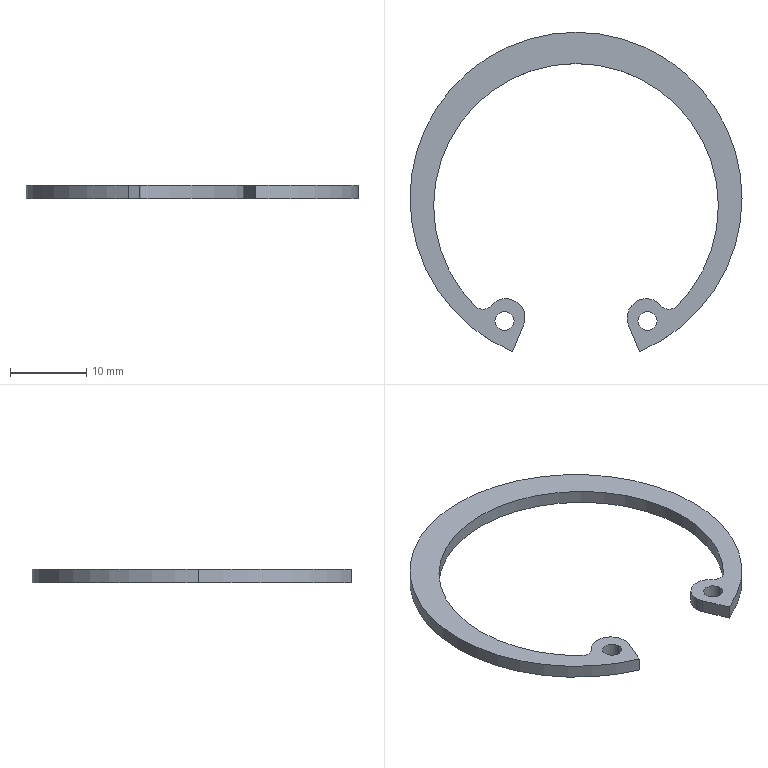Part | SolidWorks | features Extrusion 1 | 1 solid | 19 faces | box 43.5 x 41.844 x 1.75 mm | volume 670.953 mm3 | cylinder 15 | plane 4 | commonest cylinder face diameters 2.5 x4 5 x3 37.3 x3 43.5 x3 3 x2
STEP:
#1=CARTESIAN_POINT('',(8.113,-16.072,1.75));
#2=VERTEX_POINT('',#1);
#3=CARTESIAN_POINT('',(10.613,-16.072,1.75));
#4=VERTEX_POINT('',#3);
#5=CARTESIAN_POINT('',(9.363,-16.072,1.75));
#6=DIRECTION('',(0.,0.,1.));
#7=DIRECTION('',(-1.,0.,0.));
#8=AXIS2_PLACEMENT_3D('',#5,#6,#7);
#9=CIRCLE('',#8,1.25);
#10=EDGE_CURVE('',#2,#4,#9,.T.);
#11=ORIENTED_EDGE('',*,*,#10,.T.);
#12=CARTESIAN_POINT('',(10.613,-16.072,0.));
#13=VERTEX_POINT('',#12);
#14=CARTESIAN_POINT('',(10.613,-16.072,1.75));
#15=DIRECTION('',(0.,0.,-1.));
#16=VECTOR('',#15,1000.);
#17=LINE('',#14,#16);
#18=EDGE_CURVE('',#4,#13,#17,.T.);
#19=ORIENTED_EDGE('',*,*,#18,.T.);
#20=CARTESIAN_POINT('',(8.113,-16.072,0.));
#21=VERTEX_POINT('',#20);
#22=CARTESIAN_POINT('',(9.363,-16.072,0.));
#23=DIRECTION('',(0.,0.,1.));
#24=DIRECTION('',(-1.,0.,0.));
#25=AXIS2_PLACEMENT_3D('',#22,#23,#24);
#26=CIRCLE('',#25,1.25);
#27=EDGE_CURVE('',#21,#13,#26,.T.);
#28=ORIENTED_EDGE('',*,*,#27,.F.);
#29=CARTESIAN_POINT('',(8.113,-16.072,1.75));
#30=DIRECTION('',(0.,0.,-1.));
#31=VECTOR('',#30,1000.);
#32=LINE('',#29,#31);
#33=EDGE_CURVE('',#2,#21,#32,.T.);
#34=ORIENTED_EDGE('',*,*,#33,.F.);
#35=EDGE_LOOP('',(#11,#19,#28,#34));
#36=FACE_OUTER_BOUND('',#35,.T.);
#37=CARTESIAN_POINT('',(9.363,-16.072,1.75));
#38=DIRECTION('',(0.,0.,-1.));
#39=DIRECTION('',(-1.,0.,0.));
#40=AXIS2_PLACEMENT_3D('',#37,#38,#39);
#41=CYLINDRICAL_SURFACE('',#40,1.25);
#42=ADVANCED_FACE('',(#36),#41,.F.);
#43=CARTESIAN_POINT('',(-10.613,-16.072,1.75));
#44=VERTEX_POINT('',#43);
#45=CARTESIAN_POINT('',(-8.113,-16.072,1.75));
#46=VERTEX_POINT('',#45);
#47=CARTESIAN_POINT('',(-9.363,-16.072,1.75));
#48=DIRECTION('',(0.,0.,1.));
#49=DIRECTION('',(1.,0.,0.));
#50=AXIS2_PLACEMENT_3D('',#47,#48,#49);
#51=CIRCLE('',#50,1.25);
#52=EDGE_CURVE('',#44,#46,#51,.T.);
#53=ORIENTED_EDGE('',*,*,#52,.T.);
#54=CARTESIAN_POINT('',(-8.113,-16.072,0.));
#55=VERTEX_POINT('',#54);
#56=CARTESIAN_POINT('',(-8.113,-16.072,1.75));
#57=DIRECTION('',(0.,0.,-1.));
#58=VECTOR('',#57,1000.);
#59=LINE('',#56,#58);
#60=EDGE_CURVE('',#46,#55,#59,.T.);
#61=ORIENTED_EDGE('',*,*,#60,.T.);
#62=CARTESIAN_POINT('',(-10.613,-16.072,0.));
#63=VERTEX_POINT('',#62);
#64=CARTESIAN_POINT('',(-9.363,-16.072,0.));
#65=DIRECTION('',(0.,0.,1.));
#66=DIRECTION('',(1.,0.,0.));
#67=AXIS2_PLACEMENT_3D('',#64,#65,#66);
#68=CIRCLE('',#67,1.25);
#69=EDGE_CURVE('',#63,#55,#68,.T.);
#70=ORIENTED_EDGE('',*,*,#69,.F.);
#71=CARTESIAN_POINT('',(-10.613,-16.072,1.75));
#72=DIRECTION('',(0.,0.,-1.));
#73=VECTOR('',#72,1000.);
#74=LINE('',#71,#73);
#75=EDGE_CURVE('',#44,#63,#74,.T.);
#76=ORIENTED_EDGE('',*,*,#75,.F.);
#77=EDGE_LOOP('',(#53,#61,#70,#76));
#78=FACE_OUTER_BOUND('',#77,.T.);
#79=CARTESIAN_POINT('',(-9.363,-16.072,1.75));
#80=DIRECTION('',(0.,0.,-1.));
#81=DIRECTION('',(-1.,0.,0.));
#82=AXIS2_PLACEMENT_3D('',#79,#80,#81);
#83=CYLINDRICAL_SURFACE('',#82,1.25);
#84=ADVANCED_FACE('',(#78),#83,.F.);
#85=CARTESIAN_POINT('',(21.75,0.,1.75));
#86=VERTEX_POINT('',#85);
#87=CARTESIAN_POINT('',(-21.75,0.,1.75));
#88=VERTEX_POINT('',#87);
#89=CARTESIAN_POINT('',(0.,0.,1.75));
#90=DIRECTION('',(0.,0.,1.));
#91=DIRECTION('',(1.,0.,0.));
#92=AXIS2_PLACEMENT_3D('',#89,#90,#91);
#93=CIRCLE('',#92,21.75);
#94=EDGE_CURVE('',#86,#88,#93,.T.);
#95=ORIENTED_EDGE('',*,*,#94,.F.);
#96=CARTESIAN_POINT('',(21.75,0.,0.));
#97=VERTEX_POINT('',#96);
#98=CARTESIAN_POINT('',(21.75,0.,1.75));
#99=DIRECTION('',(0.,0.,-1.));
#100=VECTOR('',#99,1000.);
#101=LINE('',#98,#100);
#102=EDGE_CURVE('',#86,#97,#101,.T.);
#103=ORIENTED_EDGE('',*,*,#102,.T.);
#104=CARTESIAN_POINT('',(-21.75,0.,0.));
#105=VERTEX_POINT('',#104);
#106=CARTESIAN_POINT('',(0.,0.,0.));
#107=DIRECTION('',(0.,0.,1.));
#108=DIRECTION('',(1.,0.,0.));
#109=AXIS2_PLACEMENT_3D('',#106,#107,#108);
#110=CIRCLE('',#109,21.75);
#111=EDGE_CURVE('',#97,#105,#110,.T.);
#112=ORIENTED_EDGE('',*,*,#111,.T.);
#113=CARTESIAN_POINT('',(-21.75,0.,1.75));
#114=DIRECTION('',(0.,0.,-1.));
#115=VECTOR('',#114,1000.);
#116=LINE('',#113,#115);
#117=EDGE_CURVE('',#88,#105,#116,.T.);
#118=ORIENTED_EDGE('',*,*,#117,.F.);
#119=EDGE_LOOP('',(#95,#103,#112,#118));
#120=FACE_OUTER_BOUND('',#119,.T.);
#121=CARTESIAN_POINT('',(0.,0.,1.75));
#122=DIRECTION('',(0.,0.,-1.));
#123=DIRECTION('',(-1.,0.,0.));
#124=AXIS2_PLACEMENT_3D('',#121,#122,#123);
#125=CYLINDRICAL_SURFACE('',#124,21.75);
#126=ADVANCED_FACE('',(#120),#125,.T.);
#127=CARTESIAN_POINT('',(-8.323,-20.094,1.75));
#128=VERTEX_POINT('',#127);
#129=CARTESIAN_POINT('',(0.,0.,1.75));
#130=DIRECTION('',(0.,0.,1.));
#131=DIRECTION('',(1.,0.,0.));
#132=AXIS2_PLACEMENT_3D('',#129,#130,#131);
#133=CIRCLE('',#132,21.75);
#134=EDGE_CURVE('',#88,#128,#133,.T.);
#135=ORIENTED_EDGE('',*,*,#134,.F.);
#136=ORIENTED_EDGE('',*,*,#117,.T.);
#137=CARTESIAN_POINT('',(-8.323,-20.094,0.));
#138=VERTEX_POINT('',#137);
#139=CARTESIAN_POINT('',(0.,0.,0.));
#140=DIRECTION('',(0.,0.,1.));
#141=DIRECTION('',(1.,0.,0.));
#142=AXIS2_PLACEMENT_3D('',#139,#140,#141);
#143=CIRCLE('',#142,21.75);
#144=EDGE_CURVE('',#105,#138,#143,.T.);
#145=ORIENTED_EDGE('',*,*,#144,.T.);
#146=CARTESIAN_POINT('',(-8.323,-20.094,1.75));
#147=DIRECTION('',(0.,0.,-1.));
#148=VECTOR('',#147,1000.);
#149=LINE('',#146,#148);
#150=EDGE_CURVE('',#128,#138,#149,.T.);
#151=ORIENTED_EDGE('',*,*,#150,.F.);
#152=EDGE_LOOP('',(#135,#136,#145,#151));
#153=FACE_OUTER_BOUND('',#152,.T.);
#154=CARTESIAN_POINT('',(0.,0.,1.75));
#155=DIRECTION('',(0.,0.,-1.));
#156=DIRECTION('',(-1.,0.,0.));
#157=AXIS2_PLACEMENT_3D('',#154,#155,#156);
#158=CYLINDRICAL_SURFACE('',#157,21.75);
#159=ADVANCED_FACE('',(#153),#158,.T.);
#160=CARTESIAN_POINT('',(6.689,-15.652,1.75));
#161=VERTEX_POINT('',#160);
#162=CARTESIAN_POINT('',(6.879,-16.609,1.75));
#163=VERTEX_POINT('',#162);
#164=CARTESIAN_POINT('',(9.189,-15.652,1.75));
#165=DIRECTION('',(0.,0.,1.));
#166=DIRECTION('',(-1.,0.,0.));
#167=AXIS2_PLACEMENT_3D('',#164,#165,#166);
#168=CIRCLE('',#167,2.5);
#169=EDGE_CURVE('',#161,#163,#168,.T.);
#170=ORIENTED_EDGE('',*,*,#169,.F.);
#171=CARTESIAN_POINT('',(6.689,-15.652,0.));
#172=VERTEX_POINT('',#171);
#173=CARTESIAN_POINT('',(6.689,-15.652,1.75));
#174=DIRECTION('',(0.,0.,-1.));
#175=VECTOR('',#174,1000.);
#176=LINE('',#173,#175);
#177=EDGE_CURVE('',#161,#172,#176,.T.);
#178=ORIENTED_EDGE('',*,*,#177,.T.);
#179=CARTESIAN_POINT('',(6.879,-16.609,0.));
#180=VERTEX_POINT('',#179);
#181=CARTESIAN_POINT('',(9.189,-15.652,0.));
#182=DIRECTION('',(0.,0.,1.));
#183=DIRECTION('',(-1.,0.,0.));
#184=AXIS2_PLACEMENT_3D('',#181,#182,#183);
#185=CIRCLE('',#184,2.5);
#186=EDGE_CURVE('',#172,#180,#185,.T.);
#187=ORIENTED_EDGE('',*,*,#186,.T.);
#188=CARTESIAN_POINT('',(6.879,-16.609,1.75));
#189=DIRECTION('',(0.,0.,-1.));
#190=VECTOR('',#189,1000.);
#191=LINE('',#188,#190);
#192=EDGE_CURVE('',#163,#180,#191,.T.);
#193=ORIENTED_EDGE('',*,*,#192,.F.);
#194=EDGE_LOOP('',(#170,#178,#187,#193));
#195=FACE_OUTER_BOUND('',#194,.T.);
#196=CARTESIAN_POINT('',(9.189,-15.652,1.75));
#197=DIRECTION('',(0.,0.,-1.));
#198=DIRECTION('',(-1.,0.,0.));
#199=AXIS2_PLACEMENT_3D('',#196,#197,#198);
#200=CYLINDRICAL_SURFACE('',#199,2.5);
#201=ADVANCED_FACE('',(#195),#200,.T.);
#202=CARTESIAN_POINT('',(18.65,-1.,1.75));
#203=VERTEX_POINT('',#202);
#204=CARTESIAN_POINT('',(13.285,-14.09,1.75));
#205=VERTEX_POINT('',#204);
#206=CARTESIAN_POINT('',(0.,-1.,1.75));
#207=DIRECTION('',(0.,0.,-1.));
#208=DIRECTION('',(1.,0.,0.));
#209=AXIS2_PLACEMENT_3D('',#206,#207,#208);
#210=CIRCLE('',#209,18.65);
#211=EDGE_CURVE('',#203,#205,#210,.T.);
#212=ORIENTED_EDGE('',*,*,#211,.F.);
#213=CARTESIAN_POINT('',(18.65,-1.,0.));
#214=VERTEX_POINT('',#213);
#215=CARTESIAN_POINT('',(18.65,-1.,1.75));
#216=DIRECTION('',(0.,0.,-1.));
#217=VECTOR('',#216,1000.);
#218=LINE('',#215,#217);
#219=EDGE_CURVE('',#203,#214,#218,.T.);
#220=ORIENTED_EDGE('',*,*,#219,.T.);
#221=CARTESIAN_POINT('',(13.285,-14.09,0.));
#222=VERTEX_POINT('',#221);
#223=CARTESIAN_POINT('',(0.,-1.,0.));
#224=DIRECTION('',(0.,0.,-1.));
#225=DIRECTION('',(1.,0.,0.));
#226=AXIS2_PLACEMENT_3D('',#223,#224,#225);
#227=CIRCLE('',#226,18.65);
#228=EDGE_CURVE('',#214,#222,#227,.T.);
#229=ORIENTED_EDGE('',*,*,#228,.T.);
#230=CARTESIAN_POINT('',(13.285,-14.09,1.75));
#231=DIRECTION('',(0.,0.,-1.));
#232=VECTOR('',#231,1000.);
#233=LINE('',#230,#232);
#234=EDGE_CURVE('',#205,#222,#233,.T.);
#235=ORIENTED_EDGE('',*,*,#234,.F.);
#236=EDGE_LOOP('',(#212,#220,#229,#235));
#237=FACE_OUTER_BOUND('',#236,.T.);
#238=CARTESIAN_POINT('',(0.,-1.,1.75));
#239=DIRECTION('',(0.,0.,-1.));
#240=DIRECTION('',(-1.,0.,0.));
#241=AXIS2_PLACEMENT_3D('',#238,#239,#240);
#242=CYLINDRICAL_SURFACE('',#241,18.65);
#243=ADVANCED_FACE('',(#237),#242,.F.);
#244=ORIENTED_EDGE('',*,*,#219,.F.);
#245=CARTESIAN_POINT('',(-18.65,-1.,1.75));
#246=VERTEX_POINT('',#245);
#247=CARTESIAN_POINT('',(0.,-1.,1.75));
#248=DIRECTION('',(0.,0.,-1.));
#249=DIRECTION('',(1.,0.,0.));
#250=AXIS2_PLACEMENT_3D('',#247,#248,#249);
#251=CIRCLE('',#250,18.65);
#252=EDGE_CURVE('',#246,#203,#251,.T.);
#253=ORIENTED_EDGE('',*,*,#252,.F.);
#254=CARTESIAN_POINT('',(-18.65,-1.,0.));
#255=VERTEX_POINT('',#254);
#256=CARTESIAN_POINT('',(-18.65,-1.,1.75));
#257=DIRECTION('',(0.,0.,-1.));
#258=VECTOR('',#257,1000.);
#259=LINE('',#256,#258);
#260=EDGE_CURVE('',#246,#255,#259,.T.);
#261=ORIENTED_EDGE('',*,*,#260,.T.);
#262=CARTESIAN_POINT('',(0.,-1.,0.));
#263=DIRECTION('',(0.,0.,-1.));
#264=DIRECTION('',(1.,0.,0.));
#265=AXIS2_PLACEMENT_3D('',#262,#263,#264);
#266=CIRCLE('',#265,18.65);
#267=EDGE_CURVE('',#255,#214,#266,.T.);
#268=ORIENTED_EDGE('',*,*,#267,.T.);
#269=EDGE_LOOP('',(#244,#253,#261,#268));
#270=FACE_OUTER_BOUND('',#269,.T.);
#271=CARTESIAN_POINT('',(0.,-1.,1.75));
#272=DIRECTION('',(0.,0.,-1.));
#273=DIRECTION('',(-1.,0.,0.));
#274=AXIS2_PLACEMENT_3D('',#271,#272,#273);
#275=CYLINDRICAL_SURFACE('',#274,18.65);
#276=ADVANCED_FACE('',(#270),#275,.F.);
#277=ORIENTED_EDGE('',*,*,#52,.F.);
#278=CARTESIAN_POINT('',(-9.363,-16.072,1.75));
#279=DIRECTION('',(0.,0.,1.));
#280=DIRECTION('',(1.,0.,0.));
#281=AXIS2_PLACEMENT_3D('',#278,#279,#280);
#282=CIRCLE('',#281,1.25);
#283=EDGE_CURVE('',#46,#44,#282,.T.);
#284=ORIENTED_EDGE('',*,*,#283,.F.);
#285=EDGE_LOOP('',(#277,#284));
#286=FACE_BOUND('',#285,.T.);
#287=CARTESIAN_POINT('',(-6.879,-16.609,1.75));
#288=VERTEX_POINT('',#287);
#289=CARTESIAN_POINT('',(-11.081,-14.018,1.75));
#290=VERTEX_POINT('',#289);
#291=CARTESIAN_POINT('',(-9.189,-15.652,1.75));
#292=DIRECTION('',(0.,0.,1.));
#293=DIRECTION('',(1.,0.,0.));
#294=AXIS2_PLACEMENT_3D('',#291,#292,#293);
#295=CIRCLE('',#294,2.5);
#296=EDGE_CURVE('',#288,#290,#295,.T.);
#297=ORIENTED_EDGE('',*,*,#296,.T.);
#298=CARTESIAN_POINT('',(-13.285,-14.09,1.75));
#299=VERTEX_POINT('',#298);
#300=CARTESIAN_POINT('',(-12.216,-13.037,1.75));
#301=DIRECTION('',(0.,0.,-1.));
#302=DIRECTION('',(-1.,0.,0.));
#303=AXIS2_PLACEMENT_3D('',#300,#301,#302);
#304=CIRCLE('',#303,1.5);
#305=EDGE_CURVE('',#290,#299,#304,.T.);
#306=ORIENTED_EDGE('',*,*,#305,.T.);
#307=CARTESIAN_POINT('',(0.,-1.,1.75));
#308=DIRECTION('',(0.,0.,-1.));
#309=DIRECTION('',(1.,0.,0.));
#310=AXIS2_PLACEMENT_3D('',#307,#308,#309);
#311=CIRCLE('',#310,18.65);
#312=EDGE_CURVE('',#299,#246,#311,.T.);
#313=ORIENTED_EDGE('',*,*,#312,.T.);
#314=ORIENTED_EDGE('',*,*,#252,.T.);
#315=ORIENTED_EDGE('',*,*,#211,.T.);
#316=CARTESIAN_POINT('',(11.081,-14.018,1.75));
#317=VERTEX_POINT('',#316);
#318=CARTESIAN_POINT('',(12.216,-13.037,1.75));
#319=DIRECTION('',(0.,0.,-1.));
#320=DIRECTION('',(1.,0.,0.));
#321=AXIS2_PLACEMENT_3D('',#318,#319,#320);
#322=CIRCLE('',#321,1.5);
#323=EDGE_CURVE('',#205,#317,#322,.T.);
#324=ORIENTED_EDGE('',*,*,#323,.T.);
#325=CARTESIAN_POINT('',(9.189,-15.652,1.75));
#326=DIRECTION('',(0.,0.,1.));
#327=DIRECTION('',(-1.,0.,0.));
#328=AXIS2_PLACEMENT_3D('',#325,#326,#327);
#329=CIRCLE('',#328,2.5);
#330=EDGE_CURVE('',#317,#161,#329,.T.);
#331=ORIENTED_EDGE('',*,*,#330,.T.);
#332=ORIENTED_EDGE('',*,*,#169,.T.);
#333=CARTESIAN_POINT('',(8.323,-20.094,1.75));
#334=VERTEX_POINT('',#333);
#335=CARTESIAN_POINT('',(6.879,-16.609,1.75));
#336=DIRECTION('',(0.3827,-0.9239,0.));
#337=VECTOR('',#336,1000.);
#338=LINE('',#335,#337);
#339=EDGE_CURVE('',#163,#334,#338,.T.);
#340=ORIENTED_EDGE('',*,*,#339,.T.);
#341=CARTESIAN_POINT('',(0.,0.,1.75));
#342=DIRECTION('',(0.,0.,1.));
#343=DIRECTION('',(1.,0.,0.));
#344=AXIS2_PLACEMENT_3D('',#341,#342,#343);
#345=CIRCLE('',#344,21.75);
#346=EDGE_CURVE('',#334,#86,#345,.T.);
#347=ORIENTED_EDGE('',*,*,#346,.T.);
#348=ORIENTED_EDGE('',*,*,#94,.T.);
#349=ORIENTED_EDGE('',*,*,#134,.T.);
#350=CARTESIAN_POINT('',(-6.879,-16.609,1.75));
#351=DIRECTION('',(0.3827,0.9239,0.));
#352=VECTOR('',#351,1000.);
#353=LINE('',#350,#352);
#354=EDGE_CURVE('',#128,#288,#353,.T.);
#355=ORIENTED_EDGE('',*,*,#354,.T.);
#356=EDGE_LOOP('',(#297,#306,#313,#314,#315,#324,#331,#332,#340,#347,#348,#349,#355));
#357=FACE_OUTER_BOUND('',#356,.T.);
#358=ORIENTED_EDGE('',*,*,#10,.F.);
#359=CARTESIAN_POINT('',(9.363,-16.072,1.75));
#360=DIRECTION('',(0.,0.,1.));
#361=DIRECTION('',(-1.,0.,0.));
#362=AXIS2_PLACEMENT_3D('',#359,#360,#361);
#363=CIRCLE('',#362,1.25);
#364=EDGE_CURVE('',#4,#2,#363,.T.);
#365=ORIENTED_EDGE('',*,*,#364,.F.);
#366=EDGE_LOOP('',(#358,#365));
#367=FACE_BOUND('',#366,.T.);
#368=CARTESIAN_POINT('',(-9.189,-15.652,1.75));
#369=DIRECTION('',(0.,0.,1.));
#370=DIRECTION('',(1.,0.,0.));
#371=AXIS2_PLACEMENT_3D('',#368,#369,#370);
#372=PLANE('',#371);
#373=ADVANCED_FACE('',(#286,#357,#367),#372,.T.);
#374=CARTESIAN_POINT('',(-6.879,-16.609,0.));
#375=VERTEX_POINT('',#374);
#376=CARTESIAN_POINT('',(-11.081,-14.018,0.));
#377=VERTEX_POINT('',#376);
#378=CARTESIAN_POINT('',(-9.189,-15.652,0.));
#379=DIRECTION('',(0.,0.,1.));
#380=DIRECTION('',(1.,0.,0.));
#381=AXIS2_PLACEMENT_3D('',#378,#379,#380);
#382=CIRCLE('',#381,2.5);
#383=EDGE_CURVE('',#375,#377,#382,.T.);
#384=ORIENTED_EDGE('',*,*,#383,.F.);
#385=CARTESIAN_POINT('',(-6.879,-16.609,0.));
#386=DIRECTION('',(0.3827,0.9239,0.));
#387=VECTOR('',#386,1000.);
#388=LINE('',#385,#387);
#389=EDGE_CURVE('',#138,#375,#388,.T.);
#390=ORIENTED_EDGE('',*,*,#389,.F.);
#391=ORIENTED_EDGE('',*,*,#144,.F.);
#392=ORIENTED_EDGE('',*,*,#111,.F.);
#393=CARTESIAN_POINT('',(8.323,-20.094,0.));
#394=VERTEX_POINT('',#393);
#395=CARTESIAN_POINT('',(0.,0.,0.));
#396=DIRECTION('',(0.,0.,1.));
#397=DIRECTION('',(1.,0.,0.));
#398=AXIS2_PLACEMENT_3D('',#395,#396,#397);
#399=CIRCLE('',#398,21.75);
#400=EDGE_CURVE('',#394,#97,#399,.T.);
#401=ORIENTED_EDGE('',*,*,#400,.F.);
#402=CARTESIAN_POINT('',(6.879,-16.609,0.));
#403=DIRECTION('',(0.3827,-0.9239,0.));
#404=VECTOR('',#403,1000.);
#405=LINE('',#402,#404);
#406=EDGE_CURVE('',#180,#394,#405,.T.);
#407=ORIENTED_EDGE('',*,*,#406,.F.);
#408=ORIENTED_EDGE('',*,*,#186,.F.);
#409=CARTESIAN_POINT('',(11.081,-14.018,0.));
#410=VERTEX_POINT('',#409);
#411=CARTESIAN_POINT('',(9.189,-15.652,0.));
#412=DIRECTION('',(0.,0.,1.));
#413=DIRECTION('',(-1.,0.,0.));
#414=AXIS2_PLACEMENT_3D('',#411,#412,#413);
#415=CIRCLE('',#414,2.5);
#416=EDGE_CURVE('',#410,#172,#415,.T.);
#417=ORIENTED_EDGE('',*,*,#416,.F.);
#418=CARTESIAN_POINT('',(12.216,-13.037,0.));
#419=DIRECTION('',(0.,0.,-1.));
#420=DIRECTION('',(1.,0.,0.));
#421=AXIS2_PLACEMENT_3D('',#418,#419,#420);
#422=CIRCLE('',#421,1.5);
#423=EDGE_CURVE('',#222,#410,#422,.T.);
#424=ORIENTED_EDGE('',*,*,#423,.F.);
#425=ORIENTED_EDGE('',*,*,#228,.F.);
#426=ORIENTED_EDGE('',*,*,#267,.F.);
#427=CARTESIAN_POINT('',(-13.285,-14.09,0.));
#428=VERTEX_POINT('',#427);
#429=CARTESIAN_POINT('',(0.,-1.,0.));
#430=DIRECTION('',(0.,0.,-1.));
#431=DIRECTION('',(1.,0.,0.));
#432=AXIS2_PLACEMENT_3D('',#429,#430,#431);
#433=CIRCLE('',#432,18.65);
#434=EDGE_CURVE('',#428,#255,#433,.T.);
#435=ORIENTED_EDGE('',*,*,#434,.F.);
#436=CARTESIAN_POINT('',(-12.216,-13.037,0.));
#437=DIRECTION('',(0.,0.,-1.));
#438=DIRECTION('',(-1.,0.,0.));
#439=AXIS2_PLACEMENT_3D('',#436,#437,#438);
#440=CIRCLE('',#439,1.5);
#441=EDGE_CURVE('',#377,#428,#440,.T.);
#442=ORIENTED_EDGE('',*,*,#441,.F.);
#443=EDGE_LOOP('',(#384,#390,#391,#392,#401,#407,#408,#417,#424,#425,#426,#435,#442));
#444=FACE_OUTER_BOUND('',#443,.T.);
#445=ORIENTED_EDGE('',*,*,#69,.T.);
#446=CARTESIAN_POINT('',(-9.363,-16.072,0.));
#447=DIRECTION('',(0.,0.,1.));
#448=DIRECTION('',(1.,0.,0.));
#449=AXIS2_PLACEMENT_3D('',#446,#447,#448);
#450=CIRCLE('',#449,1.25);
#451=EDGE_CURVE('',#55,#63,#450,.T.);
#452=ORIENTED_EDGE('',*,*,#451,.T.);
#453=EDGE_LOOP('',(#445,#452));
#454=FACE_BOUND('',#453,.T.);
#455=ORIENTED_EDGE('',*,*,#27,.T.);
#456=CARTESIAN_POINT('',(9.363,-16.072,0.));
#457=DIRECTION('',(0.,0.,1.));
#458=DIRECTION('',(-1.,0.,0.));
#459=AXIS2_PLACEMENT_3D('',#456,#457,#458);
#460=CIRCLE('',#459,1.25);
#461=EDGE_CURVE('',#13,#21,#460,.T.);
#462=ORIENTED_EDGE('',*,*,#461,.T.);
#463=EDGE_LOOP('',(#455,#462));
#464=FACE_BOUND('',#463,.T.);
#465=CARTESIAN_POINT('',(-9.189,-15.652,0.));
#466=DIRECTION('',(0.,0.,1.));
#467=DIRECTION('',(1.,0.,0.));
#468=AXIS2_PLACEMENT_3D('',#465,#466,#467);
#469=PLANE('',#468);
#470=ADVANCED_FACE('',(#444,#454,#464),#469,.F.);
#471=ORIENTED_EDGE('',*,*,#383,.T.);
#472=CARTESIAN_POINT('',(-11.081,-14.018,1.75));
#473=DIRECTION('',(0.,0.,-1.));
#474=VECTOR('',#473,1000.);
#475=LINE('',#472,#474);
#476=EDGE_CURVE('',#290,#377,#475,.T.);
#477=ORIENTED_EDGE('',*,*,#476,.F.);
#478=ORIENTED_EDGE('',*,*,#296,.F.);
#479=CARTESIAN_POINT('',(-6.879,-16.609,1.75));
#480=DIRECTION('',(0.,0.,-1.));
#481=VECTOR('',#480,1000.);
#482=LINE('',#479,#481);
#483=EDGE_CURVE('',#288,#375,#482,.T.);
#484=ORIENTED_EDGE('',*,*,#483,.T.);
#485=EDGE_LOOP('',(#471,#477,#478,#484));
#486=FACE_OUTER_BOUND('',#485,.T.);
#487=CARTESIAN_POINT('',(-9.189,-15.652,1.75));
#488=DIRECTION('',(0.,0.,-1.));
#489=DIRECTION('',(-1.,0.,0.));
#490=AXIS2_PLACEMENT_3D('',#487,#488,#489);
#491=CYLINDRICAL_SURFACE('',#490,2.5);
#492=ADVANCED_FACE('',(#486),#491,.T.);
#493=ORIENTED_EDGE('',*,*,#441,.T.);
#494=CARTESIAN_POINT('',(-13.285,-14.09,1.75));
#495=DIRECTION('',(0.,0.,-1.));
#496=VECTOR('',#495,1000.);
#497=LINE('',#494,#496);
#498=EDGE_CURVE('',#299,#428,#497,.T.);
#499=ORIENTED_EDGE('',*,*,#498,.F.);
#500=ORIENTED_EDGE('',*,*,#305,.F.);
#501=ORIENTED_EDGE('',*,*,#476,.T.);
#502=EDGE_LOOP('',(#493,#499,#500,#501));
#503=FACE_OUTER_BOUND('',#502,.T.);
#504=CARTESIAN_POINT('',(-12.216,-13.037,1.75));
#505=DIRECTION('',(0.,0.,-1.));
#506=DIRECTION('',(-1.,0.,0.));
#507=AXIS2_PLACEMENT_3D('',#504,#505,#506);
#508=CYLINDRICAL_SURFACE('',#507,1.5);
#509=ADVANCED_FACE('',(#503),#508,.F.);
#510=ORIENTED_EDGE('',*,*,#260,.F.);
#511=ORIENTED_EDGE('',*,*,#312,.F.);
#512=ORIENTED_EDGE('',*,*,#498,.T.);
#513=ORIENTED_EDGE('',*,*,#434,.T.);
#514=EDGE_LOOP('',(#510,#511,#512,#513));
#515=FACE_OUTER_BOUND('',#514,.T.);
#516=CARTESIAN_POINT('',(0.,-1.,1.75));
#517=DIRECTION('',(0.,0.,-1.));
#518=DIRECTION('',(-1.,0.,0.));
#519=AXIS2_PLACEMENT_3D('',#516,#517,#518);
#520=CYLINDRICAL_SURFACE('',#519,18.65);
#521=ADVANCED_FACE('',(#515),#520,.F.);
#522=ORIENTED_EDGE('',*,*,#423,.T.);
#523=CARTESIAN_POINT('',(11.081,-14.018,1.75));
#524=DIRECTION('',(0.,0.,-1.));
#525=VECTOR('',#524,1000.);
#526=LINE('',#523,#525);
#527=EDGE_CURVE('',#317,#410,#526,.T.);
#528=ORIENTED_EDGE('',*,*,#527,.F.);
#529=ORIENTED_EDGE('',*,*,#323,.F.);
#530=ORIENTED_EDGE('',*,*,#234,.T.);
#531=EDGE_LOOP('',(#522,#528,#529,#530));
#532=FACE_OUTER_BOUND('',#531,.T.);
#533=CARTESIAN_POINT('',(12.216,-13.037,1.75));
#534=DIRECTION('',(0.,0.,-1.));
#535=DIRECTION('',(-1.,0.,0.));
#536=AXIS2_PLACEMENT_3D('',#533,#534,#535);
#537=CYLINDRICAL_SURFACE('',#536,1.5);
#538=ADVANCED_FACE('',(#532),#537,.F.);
#539=ORIENTED_EDGE('',*,*,#177,.F.);
#540=ORIENTED_EDGE('',*,*,#330,.F.);
#541=ORIENTED_EDGE('',*,*,#527,.T.);
#542=ORIENTED_EDGE('',*,*,#416,.T.);
#543=EDGE_LOOP('',(#539,#540,#541,#542));
#544=FACE_OUTER_BOUND('',#543,.T.);
#545=CARTESIAN_POINT('',(9.189,-15.652,1.75));
#546=DIRECTION('',(0.,0.,-1.));
#547=DIRECTION('',(-1.,0.,0.));
#548=AXIS2_PLACEMENT_3D('',#545,#546,#547);
#549=CYLINDRICAL_SURFACE('',#548,2.5);
#550=ADVANCED_FACE('',(#544),#549,.T.);
#551=ORIENTED_EDGE('',*,*,#406,.T.);
#552=CARTESIAN_POINT('',(8.323,-20.094,1.75));
#553=DIRECTION('',(0.,0.,-1.));
#554=VECTOR('',#553,1000.);
#555=LINE('',#552,#554);
#556=EDGE_CURVE('',#334,#394,#555,.T.);
#557=ORIENTED_EDGE('',*,*,#556,.F.);
#558=ORIENTED_EDGE('',*,*,#339,.F.);
#559=ORIENTED_EDGE('',*,*,#192,.T.);
#560=EDGE_LOOP('',(#551,#557,#558,#559));
#561=FACE_OUTER_BOUND('',#560,.T.);
#562=CARTESIAN_POINT('',(6.879,-16.609,1.75));
#563=DIRECTION('',(0.9239,0.3827,0.));
#564=DIRECTION('',(-0.3827,0.9239,0.));
#565=AXIS2_PLACEMENT_3D('',#562,#563,#564);
#566=PLANE('',#565);
#567=ADVANCED_FACE('',(#561),#566,.F.);
#568=ORIENTED_EDGE('',*,*,#102,.F.);
#569=ORIENTED_EDGE('',*,*,#346,.F.);
#570=ORIENTED_EDGE('',*,*,#556,.T.);
#571=ORIENTED_EDGE('',*,*,#400,.T.);
#572=EDGE_LOOP('',(#568,#569,#570,#571));
#573=FACE_OUTER_BOUND('',#572,.T.);
#574=CARTESIAN_POINT('',(0.,0.,1.75));
#575=DIRECTION('',(0.,0.,-1.));
#576=DIRECTION('',(-1.,0.,0.));
#577=AXIS2_PLACEMENT_3D('',#574,#575,#576);
#578=CYLINDRICAL_SURFACE('',#577,21.75);
#579=ADVANCED_FACE('',(#573),#578,.T.);
#580=ORIENTED_EDGE('',*,*,#389,.T.);
#581=ORIENTED_EDGE('',*,*,#483,.F.);
#582=ORIENTED_EDGE('',*,*,#354,.F.);
#583=ORIENTED_EDGE('',*,*,#150,.T.);
#584=EDGE_LOOP('',(#580,#581,#582,#583));
#585=FACE_OUTER_BOUND('',#584,.T.);
#586=CARTESIAN_POINT('',(-6.879,-16.609,1.75));
#587=DIRECTION('',(-0.9239,0.3827,0.));
#588=DIRECTION('',(-0.3827,-0.9239,0.));
#589=AXIS2_PLACEMENT_3D('',#586,#587,#588);
#590=PLANE('',#589);
#591=ADVANCED_FACE('',(#585),#590,.F.);
#592=ORIENTED_EDGE('',*,*,#60,.F.);
#593=ORIENTED_EDGE('',*,*,#283,.T.);
#594=ORIENTED_EDGE('',*,*,#75,.T.);
#595=ORIENTED_EDGE('',*,*,#451,.F.);
#596=EDGE_LOOP('',(#592,#593,#594,#595));
#597=FACE_OUTER_BOUND('',#596,.T.);
#598=CARTESIAN_POINT('',(-9.363,-16.072,1.75));
#599=DIRECTION('',(0.,0.,-1.));
#600=DIRECTION('',(-1.,0.,0.));
#601=AXIS2_PLACEMENT_3D('',#598,#599,#600);
#602=CYLINDRICAL_SURFACE('',#601,1.25);
#603=ADVANCED_FACE('',(#597),#602,.F.);
#604=ORIENTED_EDGE('',*,*,#18,.F.);
#605=ORIENTED_EDGE('',*,*,#364,.T.);
#606=ORIENTED_EDGE('',*,*,#33,.T.);
#607=ORIENTED_EDGE('',*,*,#461,.F.);
#608=EDGE_LOOP('',(#604,#605,#606,#607));
#609=FACE_OUTER_BOUND('',#608,.T.);
#610=CARTESIAN_POINT('',(9.363,-16.072,1.75));
#611=DIRECTION('',(0.,0.,-1.));
#612=DIRECTION('',(-1.,0.,0.));
#613=AXIS2_PLACEMENT_3D('',#610,#611,#612);
#614=CYLINDRICAL_SURFACE('',#613,1.25);
#615=ADVANCED_FACE('',(#609),#614,.F.);
#616=CLOSED_SHELL('',(#42,#84,#126,#159,#201,#243,#276,#373,#470,#492,#509,#521,#538,#550,#567,#579,#591,#603,#615));
#617=MANIFOLD_SOLID_BREP('',#616);
#618=CARTESIAN_POINT('',(0.,0.,0.));
#619=DIRECTION('',(0.,0.,1.));
#620=DIRECTION('',(1.,0.,0.));
#621=AXIS2_PLACEMENT_3D('',#618,#619,#620);
#622=(LENGTH_UNIT()NAMED_UNIT(*)SI_UNIT(.MILLI.,.METRE.));
#623=UNCERTAINTY_MEASURE_WITH_UNIT(LENGTH_MEASURE(0.00001),#622,'','');
#624=(NAMED_UNIT(*)PLANE_ANGLE_UNIT()SI_UNIT($,.RADIAN.));
#625=(NAMED_UNIT(*)SI_UNIT($,.STERADIAN.)SOLID_ANGLE_UNIT());
#626=(GEOMETRIC_REPRESENTATION_CONTEXT(3)GLOBAL_UNCERTAINTY_ASSIGNED_CONTEXT((#623))GLOBAL_UNIT_ASSIGNED_CONTEXT((#622,#624,#625))REPRESENTATION_CONTEXT('',''));
#627=ADVANCED_BREP_SHAPE_REPRESENTATION('',(#617,#621),#626);